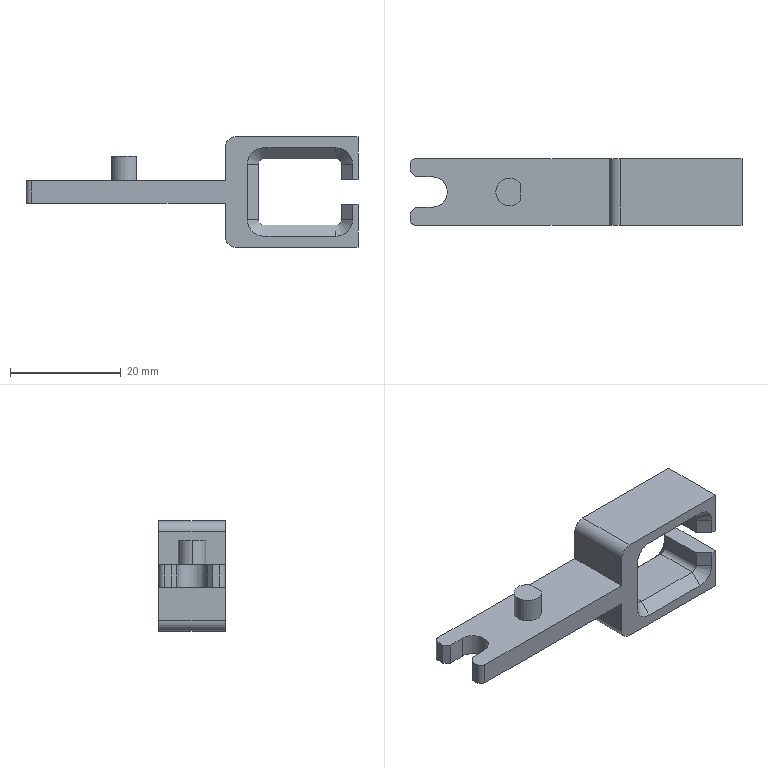Part | STEP file | Pull piece_default | 1 solid | 58 faces | box 60 x 12 x 20 mm | volume 4860 mm3 | plane 35 | cylinder 13 | cone 10 | commonest cylinder face diameters 2 x6 2.5 x2 4 x2 5 x2 5.5 x1